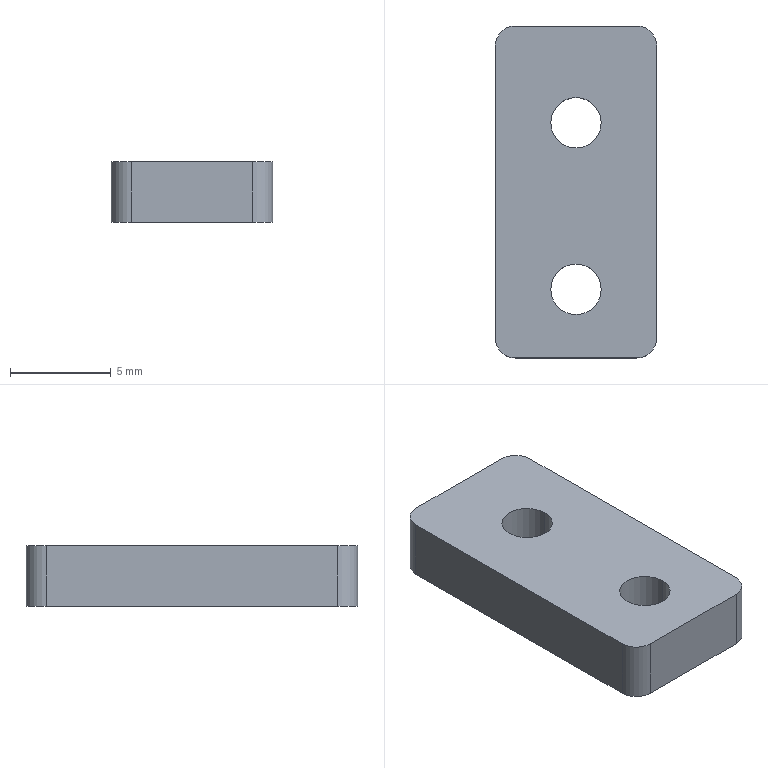Part | SolidWorks | features Extrusion 1, Fillet 1 | 1 solid | 14 faces | box 8 x 16.45 x 3 mm | volume 362.772 mm3 | cylinder 8 | plane 6 | commonest cylinder face diameters 2 x4 2.5 x4
STEP:
#1=CARTESIAN_POINT('',(-1.25,8.25,3.));
#2=VERTEX_POINT('',#1);
#3=CARTESIAN_POINT('',(1.25,8.25,3.));
#4=VERTEX_POINT('',#3);
#5=CARTESIAN_POINT('',(0.,8.25,3.));
#6=DIRECTION('',(0.,0.,1.));
#7=DIRECTION('',(1.,0.,0.));
#8=AXIS2_PLACEMENT_3D('',#5,#6,#7);
#9=CIRCLE('',#8,1.25);
#10=EDGE_CURVE('',#2,#4,#9,.T.);
#11=ORIENTED_EDGE('',*,*,#10,.T.);
#12=CARTESIAN_POINT('',(1.25,8.25,0.));
#13=VERTEX_POINT('',#12);
#14=CARTESIAN_POINT('',(1.25,8.25,3.));
#15=DIRECTION('',(0.,0.,-1.));
#16=VECTOR('',#15,1000.);
#17=LINE('',#14,#16);
#18=EDGE_CURVE('',#4,#13,#17,.T.);
#19=ORIENTED_EDGE('',*,*,#18,.T.);
#20=CARTESIAN_POINT('',(-1.25,8.25,0.));
#21=VERTEX_POINT('',#20);
#22=CARTESIAN_POINT('',(0.,8.25,0.));
#23=DIRECTION('',(0.,0.,1.));
#24=DIRECTION('',(1.,0.,0.));
#25=AXIS2_PLACEMENT_3D('',#22,#23,#24);
#26=CIRCLE('',#25,1.25);
#27=EDGE_CURVE('',#21,#13,#26,.T.);
#28=ORIENTED_EDGE('',*,*,#27,.F.);
#29=CARTESIAN_POINT('',(-1.25,8.25,3.));
#30=DIRECTION('',(0.,0.,-1.));
#31=VECTOR('',#30,1000.);
#32=LINE('',#29,#31);
#33=EDGE_CURVE('',#2,#21,#32,.T.);
#34=ORIENTED_EDGE('',*,*,#33,.F.);
#35=EDGE_LOOP('',(#11,#19,#28,#34));
#36=FACE_OUTER_BOUND('',#35,.T.);
#37=CARTESIAN_POINT('',(0.,8.25,3.));
#38=DIRECTION('',(0.,0.,-1.));
#39=DIRECTION('',(-1.,0.,0.));
#40=AXIS2_PLACEMENT_3D('',#37,#38,#39);
#41=CYLINDRICAL_SURFACE('',#40,1.25);
#42=ADVANCED_FACE('',(#36),#41,.F.);
#43=CARTESIAN_POINT('',(-1.25,0.,3.));
#44=VERTEX_POINT('',#43);
#45=CARTESIAN_POINT('',(1.25,0.,3.));
#46=VERTEX_POINT('',#45);
#47=CARTESIAN_POINT('',(0.,0.,3.));
#48=DIRECTION('',(0.,0.,1.));
#49=DIRECTION('',(1.,0.,0.));
#50=AXIS2_PLACEMENT_3D('',#47,#48,#49);
#51=CIRCLE('',#50,1.25);
#52=EDGE_CURVE('',#44,#46,#51,.T.);
#53=ORIENTED_EDGE('',*,*,#52,.T.);
#54=CARTESIAN_POINT('',(1.25,0.,0.));
#55=VERTEX_POINT('',#54);
#56=CARTESIAN_POINT('',(1.25,0.,3.));
#57=DIRECTION('',(0.,0.,-1.));
#58=VECTOR('',#57,1000.);
#59=LINE('',#56,#58);
#60=EDGE_CURVE('',#46,#55,#59,.T.);
#61=ORIENTED_EDGE('',*,*,#60,.T.);
#62=CARTESIAN_POINT('',(-1.25,0.,0.));
#63=VERTEX_POINT('',#62);
#64=CARTESIAN_POINT('',(0.,0.,0.));
#65=DIRECTION('',(0.,0.,1.));
#66=DIRECTION('',(1.,0.,0.));
#67=AXIS2_PLACEMENT_3D('',#64,#65,#66);
#68=CIRCLE('',#67,1.25);
#69=EDGE_CURVE('',#63,#55,#68,.T.);
#70=ORIENTED_EDGE('',*,*,#69,.F.);
#71=CARTESIAN_POINT('',(-1.25,0.,3.));
#72=DIRECTION('',(0.,0.,-1.));
#73=VECTOR('',#72,1000.);
#74=LINE('',#71,#73);
#75=EDGE_CURVE('',#44,#63,#74,.T.);
#76=ORIENTED_EDGE('',*,*,#75,.F.);
#77=EDGE_LOOP('',(#53,#61,#70,#76));
#78=FACE_OUTER_BOUND('',#77,.T.);
#79=CARTESIAN_POINT('',(0.,0.,3.));
#80=DIRECTION('',(0.,0.,-1.));
#81=DIRECTION('',(-1.,0.,0.));
#82=AXIS2_PLACEMENT_3D('',#79,#80,#81);
#83=CYLINDRICAL_SURFACE('',#82,1.25);
#84=ADVANCED_FACE('',(#78),#83,.F.);
#85=ORIENTED_EDGE('',*,*,#52,.F.);
#86=CARTESIAN_POINT('',(0.,0.,3.));
#87=DIRECTION('',(0.,0.,1.));
#88=DIRECTION('',(1.,0.,0.));
#89=AXIS2_PLACEMENT_3D('',#86,#87,#88);
#90=CIRCLE('',#89,1.25);
#91=EDGE_CURVE('',#46,#44,#90,.T.);
#92=ORIENTED_EDGE('',*,*,#91,.F.);
#93=EDGE_LOOP('',(#85,#92));
#94=FACE_BOUND('',#93,.T.);
#95=CARTESIAN_POINT('',(-4.,12.05,3.));
#96=VERTEX_POINT('',#95);
#97=CARTESIAN_POINT('',(-4.,-2.4,3.));
#98=VERTEX_POINT('',#97);
#99=CARTESIAN_POINT('',(-4.,13.05,3.));
#100=DIRECTION('',(0.,-1.,0.));
#101=VECTOR('',#100,1000.);
#102=LINE('',#99,#101);
#103=EDGE_CURVE('',#96,#98,#102,.T.);
#104=ORIENTED_EDGE('',*,*,#103,.T.);
#105=CARTESIAN_POINT('',(-3.,-3.4,3.));
#106=VERTEX_POINT('',#105);
#107=CARTESIAN_POINT('',(-3.,-2.4,3.));
#108=DIRECTION('',(0.,0.,1.));
#109=DIRECTION('',(1.,0.,0.));
#110=AXIS2_PLACEMENT_3D('',#107,#108,#109);
#111=CIRCLE('',#110,1.);
#112=EDGE_CURVE('',#98,#106,#111,.T.);
#113=ORIENTED_EDGE('',*,*,#112,.T.);
#114=CARTESIAN_POINT('',(3.,-3.4,3.));
#115=VERTEX_POINT('',#114);
#116=CARTESIAN_POINT('',(-4.,-3.4,3.));
#117=DIRECTION('',(1.,0.,0.));
#118=VECTOR('',#117,1000.);
#119=LINE('',#116,#118);
#120=EDGE_CURVE('',#106,#115,#119,.T.);
#121=ORIENTED_EDGE('',*,*,#120,.T.);
#122=CARTESIAN_POINT('',(4.,-2.4,3.));
#123=VERTEX_POINT('',#122);
#124=CARTESIAN_POINT('',(3.,-2.4,3.));
#125=DIRECTION('',(0.,0.,1.));
#126=DIRECTION('',(1.,0.,0.));
#127=AXIS2_PLACEMENT_3D('',#124,#125,#126);
#128=CIRCLE('',#127,1.);
#129=EDGE_CURVE('',#115,#123,#128,.T.);
#130=ORIENTED_EDGE('',*,*,#129,.T.);
#131=CARTESIAN_POINT('',(4.,12.05,3.));
#132=VERTEX_POINT('',#131);
#133=CARTESIAN_POINT('',(4.,13.05,3.));
#134=DIRECTION('',(0.,1.,0.));
#135=VECTOR('',#134,1000.);
#136=LINE('',#133,#135);
#137=EDGE_CURVE('',#123,#132,#136,.T.);
#138=ORIENTED_EDGE('',*,*,#137,.T.);
#139=CARTESIAN_POINT('',(3.,13.05,3.));
#140=VERTEX_POINT('',#139);
#141=CARTESIAN_POINT('',(3.,12.05,3.));
#142=DIRECTION('',(0.,0.,1.));
#143=DIRECTION('',(1.,0.,0.));
#144=AXIS2_PLACEMENT_3D('',#141,#142,#143);
#145=CIRCLE('',#144,1.);
#146=EDGE_CURVE('',#132,#140,#145,.T.);
#147=ORIENTED_EDGE('',*,*,#146,.T.);
#148=CARTESIAN_POINT('',(-3.,13.05,3.));
#149=VERTEX_POINT('',#148);
#150=CARTESIAN_POINT('',(-4.,13.05,3.));
#151=DIRECTION('',(-1.,0.,0.));
#152=VECTOR('',#151,1000.);
#153=LINE('',#150,#152);
#154=EDGE_CURVE('',#140,#149,#153,.T.);
#155=ORIENTED_EDGE('',*,*,#154,.T.);
#156=CARTESIAN_POINT('',(-3.,12.05,3.));
#157=DIRECTION('',(0.,0.,1.));
#158=DIRECTION('',(1.,0.,0.));
#159=AXIS2_PLACEMENT_3D('',#156,#157,#158);
#160=CIRCLE('',#159,1.);
#161=EDGE_CURVE('',#149,#96,#160,.T.);
#162=ORIENTED_EDGE('',*,*,#161,.T.);
#163=EDGE_LOOP('',(#104,#113,#121,#130,#138,#147,#155,#162));
#164=FACE_OUTER_BOUND('',#163,.T.);
#165=ORIENTED_EDGE('',*,*,#10,.F.);
#166=CARTESIAN_POINT('',(0.,8.25,3.));
#167=DIRECTION('',(0.,0.,1.));
#168=DIRECTION('',(1.,0.,0.));
#169=AXIS2_PLACEMENT_3D('',#166,#167,#168);
#170=CIRCLE('',#169,1.25);
#171=EDGE_CURVE('',#4,#2,#170,.T.);
#172=ORIENTED_EDGE('',*,*,#171,.F.);
#173=EDGE_LOOP('',(#165,#172));
#174=FACE_BOUND('',#173,.T.);
#175=CARTESIAN_POINT('',(0.,0.,3.));
#176=DIRECTION('',(0.,0.,1.));
#177=DIRECTION('',(1.,0.,0.));
#178=AXIS2_PLACEMENT_3D('',#175,#176,#177);
#179=PLANE('',#178);
#180=ADVANCED_FACE('',(#94,#164,#174),#179,.T.);
#181=CARTESIAN_POINT('',(-3.,-3.4,0.));
#182=VERTEX_POINT('',#181);
#183=CARTESIAN_POINT('',(3.,-3.4,0.));
#184=VERTEX_POINT('',#183);
#185=CARTESIAN_POINT('',(-4.,-3.4,0.));
#186=DIRECTION('',(1.,0.,0.));
#187=VECTOR('',#186,1000.);
#188=LINE('',#185,#187);
#189=EDGE_CURVE('',#182,#184,#188,.T.);
#190=ORIENTED_EDGE('',*,*,#189,.F.);
#191=CARTESIAN_POINT('',(-4.,-2.4,0.));
#192=VERTEX_POINT('',#191);
#193=CARTESIAN_POINT('',(-3.,-2.4,0.));
#194=DIRECTION('',(0.,0.,-1.));
#195=DIRECTION('',(1.,0.,0.));
#196=AXIS2_PLACEMENT_3D('',#193,#194,#195);
#197=CIRCLE('',#196,1.);
#198=EDGE_CURVE('',#182,#192,#197,.T.);
#199=ORIENTED_EDGE('',*,*,#198,.T.);
#200=CARTESIAN_POINT('',(-4.,12.05,0.));
#201=VERTEX_POINT('',#200);
#202=CARTESIAN_POINT('',(-4.,13.05,0.));
#203=DIRECTION('',(0.,-1.,0.));
#204=VECTOR('',#203,1000.);
#205=LINE('',#202,#204);
#206=EDGE_CURVE('',#201,#192,#205,.T.);
#207=ORIENTED_EDGE('',*,*,#206,.F.);
#208=CARTESIAN_POINT('',(-3.,13.05,0.));
#209=VERTEX_POINT('',#208);
#210=CARTESIAN_POINT('',(-3.,12.05,0.));
#211=DIRECTION('',(0.,0.,-1.));
#212=DIRECTION('',(1.,0.,0.));
#213=AXIS2_PLACEMENT_3D('',#210,#211,#212);
#214=CIRCLE('',#213,1.);
#215=EDGE_CURVE('',#201,#209,#214,.T.);
#216=ORIENTED_EDGE('',*,*,#215,.T.);
#217=CARTESIAN_POINT('',(3.,13.05,0.));
#218=VERTEX_POINT('',#217);
#219=CARTESIAN_POINT('',(-4.,13.05,0.));
#220=DIRECTION('',(-1.,0.,0.));
#221=VECTOR('',#220,1000.);
#222=LINE('',#219,#221);
#223=EDGE_CURVE('',#218,#209,#222,.T.);
#224=ORIENTED_EDGE('',*,*,#223,.F.);
#225=CARTESIAN_POINT('',(4.,12.05,0.));
#226=VERTEX_POINT('',#225);
#227=CARTESIAN_POINT('',(3.,12.05,0.));
#228=DIRECTION('',(0.,0.,-1.));
#229=DIRECTION('',(1.,0.,0.));
#230=AXIS2_PLACEMENT_3D('',#227,#228,#229);
#231=CIRCLE('',#230,1.);
#232=EDGE_CURVE('',#218,#226,#231,.T.);
#233=ORIENTED_EDGE('',*,*,#232,.T.);
#234=CARTESIAN_POINT('',(4.,-2.4,0.));
#235=VERTEX_POINT('',#234);
#236=CARTESIAN_POINT('',(4.,13.05,0.));
#237=DIRECTION('',(0.,1.,0.));
#238=VECTOR('',#237,1000.);
#239=LINE('',#236,#238);
#240=EDGE_CURVE('',#235,#226,#239,.T.);
#241=ORIENTED_EDGE('',*,*,#240,.F.);
#242=CARTESIAN_POINT('',(3.,-2.4,0.));
#243=DIRECTION('',(0.,0.,-1.));
#244=DIRECTION('',(1.,0.,0.));
#245=AXIS2_PLACEMENT_3D('',#242,#243,#244);
#246=CIRCLE('',#245,1.);
#247=EDGE_CURVE('',#235,#184,#246,.T.);
#248=ORIENTED_EDGE('',*,*,#247,.T.);
#249=EDGE_LOOP('',(#190,#199,#207,#216,#224,#233,#241,#248));
#250=FACE_OUTER_BOUND('',#249,.T.);
#251=ORIENTED_EDGE('',*,*,#69,.T.);
#252=CARTESIAN_POINT('',(0.,0.,0.));
#253=DIRECTION('',(0.,0.,1.));
#254=DIRECTION('',(1.,0.,0.));
#255=AXIS2_PLACEMENT_3D('',#252,#253,#254);
#256=CIRCLE('',#255,1.25);
#257=EDGE_CURVE('',#55,#63,#256,.T.);
#258=ORIENTED_EDGE('',*,*,#257,.T.);
#259=EDGE_LOOP('',(#251,#258));
#260=FACE_BOUND('',#259,.T.);
#261=ORIENTED_EDGE('',*,*,#27,.T.);
#262=CARTESIAN_POINT('',(0.,8.25,0.));
#263=DIRECTION('',(0.,0.,1.));
#264=DIRECTION('',(1.,0.,0.));
#265=AXIS2_PLACEMENT_3D('',#262,#263,#264);
#266=CIRCLE('',#265,1.25);
#267=EDGE_CURVE('',#13,#21,#266,.T.);
#268=ORIENTED_EDGE('',*,*,#267,.T.);
#269=EDGE_LOOP('',(#261,#268));
#270=FACE_BOUND('',#269,.T.);
#271=CARTESIAN_POINT('',(0.,0.,0.));
#272=DIRECTION('',(0.,0.,1.));
#273=DIRECTION('',(1.,0.,0.));
#274=AXIS2_PLACEMENT_3D('',#271,#272,#273);
#275=PLANE('',#274);
#276=ADVANCED_FACE('',(#250,#260,#270),#275,.F.);
#277=ORIENTED_EDGE('',*,*,#240,.T.);
#278=CARTESIAN_POINT('',(4.,12.05,3.));
#279=DIRECTION('',(0.,0.,1.));
#280=VECTOR('',#279,1000.);
#281=LINE('',#278,#280);
#282=EDGE_CURVE('',#226,#132,#281,.T.);
#283=ORIENTED_EDGE('',*,*,#282,.T.);
#284=ORIENTED_EDGE('',*,*,#137,.F.);
#285=CARTESIAN_POINT('',(4.,-2.4,3.));
#286=DIRECTION('',(0.,0.,-1.));
#287=VECTOR('',#286,1000.);
#288=LINE('',#285,#287);
#289=EDGE_CURVE('',#123,#235,#288,.T.);
#290=ORIENTED_EDGE('',*,*,#289,.T.);
#291=EDGE_LOOP('',(#277,#283,#284,#290));
#292=FACE_OUTER_BOUND('',#291,.T.);
#293=CARTESIAN_POINT('',(4.,13.05,3.));
#294=DIRECTION('',(-1.,0.,0.));
#295=DIRECTION('',(0.,0.,1.));
#296=AXIS2_PLACEMENT_3D('',#293,#294,#295);
#297=PLANE('',#296);
#298=ADVANCED_FACE('',(#292),#297,.F.);
#299=ORIENTED_EDGE('',*,*,#223,.T.);
#300=CARTESIAN_POINT('',(-3.,13.05,3.));
#301=DIRECTION('',(0.,0.,1.));
#302=VECTOR('',#301,1000.);
#303=LINE('',#300,#302);
#304=EDGE_CURVE('',#209,#149,#303,.T.);
#305=ORIENTED_EDGE('',*,*,#304,.T.);
#306=ORIENTED_EDGE('',*,*,#154,.F.);
#307=CARTESIAN_POINT('',(3.,13.05,3.));
#308=DIRECTION('',(0.,0.,-1.));
#309=VECTOR('',#308,1000.);
#310=LINE('',#307,#309);
#311=EDGE_CURVE('',#140,#218,#310,.T.);
#312=ORIENTED_EDGE('',*,*,#311,.T.);
#313=EDGE_LOOP('',(#299,#305,#306,#312));
#314=FACE_OUTER_BOUND('',#313,.T.);
#315=CARTESIAN_POINT('',(-4.,13.05,3.));
#316=DIRECTION('',(0.,-1.,0.));
#317=DIRECTION('',(0.,0.,-1.));
#318=AXIS2_PLACEMENT_3D('',#315,#316,#317);
#319=PLANE('',#318);
#320=ADVANCED_FACE('',(#314),#319,.F.);
#321=ORIENTED_EDGE('',*,*,#206,.T.);
#322=CARTESIAN_POINT('',(-4.,-2.4,3.));
#323=DIRECTION('',(0.,0.,1.));
#324=VECTOR('',#323,1000.);
#325=LINE('',#322,#324);
#326=EDGE_CURVE('',#192,#98,#325,.T.);
#327=ORIENTED_EDGE('',*,*,#326,.T.);
#328=ORIENTED_EDGE('',*,*,#103,.F.);
#329=CARTESIAN_POINT('',(-4.,12.05,3.));
#330=DIRECTION('',(0.,0.,-1.));
#331=VECTOR('',#330,1000.);
#332=LINE('',#329,#331);
#333=EDGE_CURVE('',#96,#201,#332,.T.);
#334=ORIENTED_EDGE('',*,*,#333,.T.);
#335=EDGE_LOOP('',(#321,#327,#328,#334));
#336=FACE_OUTER_BOUND('',#335,.T.);
#337=CARTESIAN_POINT('',(-4.,13.05,3.));
#338=DIRECTION('',(1.,0.,0.));
#339=DIRECTION('',(0.,1.,0.));
#340=AXIS2_PLACEMENT_3D('',#337,#338,#339);
#341=PLANE('',#340);
#342=ADVANCED_FACE('',(#336),#341,.F.);
#343=ORIENTED_EDGE('',*,*,#120,.F.);
#344=CARTESIAN_POINT('',(-3.,-3.4,3.));
#345=DIRECTION('',(0.,0.,-1.));
#346=VECTOR('',#345,1000.);
#347=LINE('',#344,#346);
#348=EDGE_CURVE('',#106,#182,#347,.T.);
#349=ORIENTED_EDGE('',*,*,#348,.T.);
#350=ORIENTED_EDGE('',*,*,#189,.T.);
#351=CARTESIAN_POINT('',(3.,-3.4,3.));
#352=DIRECTION('',(0.,0.,1.));
#353=VECTOR('',#352,1000.);
#354=LINE('',#351,#353);
#355=EDGE_CURVE('',#184,#115,#354,.T.);
#356=ORIENTED_EDGE('',*,*,#355,.T.);
#357=EDGE_LOOP('',(#343,#349,#350,#356));
#358=FACE_OUTER_BOUND('',#357,.T.);
#359=CARTESIAN_POINT('',(-4.,-3.4,3.));
#360=DIRECTION('',(0.,1.,0.));
#361=DIRECTION('',(0.,0.,1.));
#362=AXIS2_PLACEMENT_3D('',#359,#360,#361);
#363=PLANE('',#362);
#364=ADVANCED_FACE('',(#358),#363,.F.);
#365=ORIENTED_EDGE('',*,*,#60,.F.);
#366=ORIENTED_EDGE('',*,*,#91,.T.);
#367=ORIENTED_EDGE('',*,*,#75,.T.);
#368=ORIENTED_EDGE('',*,*,#257,.F.);
#369=EDGE_LOOP('',(#365,#366,#367,#368));
#370=FACE_OUTER_BOUND('',#369,.T.);
#371=CARTESIAN_POINT('',(0.,0.,3.));
#372=DIRECTION('',(0.,0.,-1.));
#373=DIRECTION('',(-1.,0.,0.));
#374=AXIS2_PLACEMENT_3D('',#371,#372,#373);
#375=CYLINDRICAL_SURFACE('',#374,1.25);
#376=ADVANCED_FACE('',(#370),#375,.F.);
#377=ORIENTED_EDGE('',*,*,#18,.F.);
#378=ORIENTED_EDGE('',*,*,#171,.T.);
#379=ORIENTED_EDGE('',*,*,#33,.T.);
#380=ORIENTED_EDGE('',*,*,#267,.F.);
#381=EDGE_LOOP('',(#377,#378,#379,#380));
#382=FACE_OUTER_BOUND('',#381,.T.);
#383=CARTESIAN_POINT('',(0.,8.25,3.));
#384=DIRECTION('',(0.,0.,-1.));
#385=DIRECTION('',(-1.,0.,0.));
#386=AXIS2_PLACEMENT_3D('',#383,#384,#385);
#387=CYLINDRICAL_SURFACE('',#386,1.25);
#388=ADVANCED_FACE('',(#382),#387,.F.);
#389=ORIENTED_EDGE('',*,*,#112,.F.);
#390=ORIENTED_EDGE('',*,*,#326,.F.);
#391=ORIENTED_EDGE('',*,*,#198,.F.);
#392=ORIENTED_EDGE('',*,*,#348,.F.);
#393=EDGE_LOOP('',(#389,#390,#391,#392));
#394=FACE_OUTER_BOUND('',#393,.T.);
#395=CARTESIAN_POINT('',(-3.,-2.4,3.));
#396=DIRECTION('',(0.,0.,-1.));
#397=DIRECTION('',(-1.,0.,0.));
#398=AXIS2_PLACEMENT_3D('',#395,#396,#397);
#399=CYLINDRICAL_SURFACE('',#398,1.);
#400=ADVANCED_FACE('',(#394),#399,.T.);
#401=ORIENTED_EDGE('',*,*,#161,.F.);
#402=ORIENTED_EDGE('',*,*,#304,.F.);
#403=ORIENTED_EDGE('',*,*,#215,.F.);
#404=ORIENTED_EDGE('',*,*,#333,.F.);
#405=EDGE_LOOP('',(#401,#402,#403,#404));
#406=FACE_OUTER_BOUND('',#405,.T.);
#407=CARTESIAN_POINT('',(-3.,12.05,3.));
#408=DIRECTION('',(0.,0.,-1.));
#409=DIRECTION('',(-1.,0.,0.));
#410=AXIS2_PLACEMENT_3D('',#407,#408,#409);
#411=CYLINDRICAL_SURFACE('',#410,1.);
#412=ADVANCED_FACE('',(#406),#411,.T.);
#413=ORIENTED_EDGE('',*,*,#146,.F.);
#414=ORIENTED_EDGE('',*,*,#282,.F.);
#415=ORIENTED_EDGE('',*,*,#232,.F.);
#416=ORIENTED_EDGE('',*,*,#311,.F.);
#417=EDGE_LOOP('',(#413,#414,#415,#416));
#418=FACE_OUTER_BOUND('',#417,.T.);
#419=CARTESIAN_POINT('',(3.,12.05,3.));
#420=DIRECTION('',(0.,0.,-1.));
#421=DIRECTION('',(-1.,0.,0.));
#422=AXIS2_PLACEMENT_3D('',#419,#420,#421);
#423=CYLINDRICAL_SURFACE('',#422,1.);
#424=ADVANCED_FACE('',(#418),#423,.T.);
#425=ORIENTED_EDGE('',*,*,#129,.F.);
#426=ORIENTED_EDGE('',*,*,#355,.F.);
#427=ORIENTED_EDGE('',*,*,#247,.F.);
#428=ORIENTED_EDGE('',*,*,#289,.F.);
#429=EDGE_LOOP('',(#425,#426,#427,#428));
#430=FACE_OUTER_BOUND('',#429,.T.);
#431=CARTESIAN_POINT('',(3.,-2.4,3.));
#432=DIRECTION('',(0.,0.,-1.));
#433=DIRECTION('',(-1.,0.,0.));
#434=AXIS2_PLACEMENT_3D('',#431,#432,#433);
#435=CYLINDRICAL_SURFACE('',#434,1.);
#436=ADVANCED_FACE('',(#430),#435,.T.);
#437=CLOSED_SHELL('',(#42,#84,#180,#276,#298,#320,#342,#364,#376,#388,#400,#412,#424,#436));
#438=MANIFOLD_SOLID_BREP('',#437);
#439=CARTESIAN_POINT('',(0.,0.,0.));
#440=DIRECTION('',(0.,0.,1.));
#441=DIRECTION('',(1.,0.,0.));
#442=AXIS2_PLACEMENT_3D('',#439,#440,#441);
#443=(LENGTH_UNIT()NAMED_UNIT(*)SI_UNIT(.MILLI.,.METRE.));
#444=UNCERTAINTY_MEASURE_WITH_UNIT(LENGTH_MEASURE(0.00001),#443,'','');
#445=(NAMED_UNIT(*)PLANE_ANGLE_UNIT()SI_UNIT($,.RADIAN.));
#446=(NAMED_UNIT(*)SI_UNIT($,.STERADIAN.)SOLID_ANGLE_UNIT());
#447=(GEOMETRIC_REPRESENTATION_CONTEXT(3)GLOBAL_UNCERTAINTY_ASSIGNED_CONTEXT((#444))GLOBAL_UNIT_ASSIGNED_CONTEXT((#443,#445,#446))REPRESENTATION_CONTEXT('',''));
#448=ADVANCED_BREP_SHAPE_REPRESENTATION('',(#438,#442),#447);